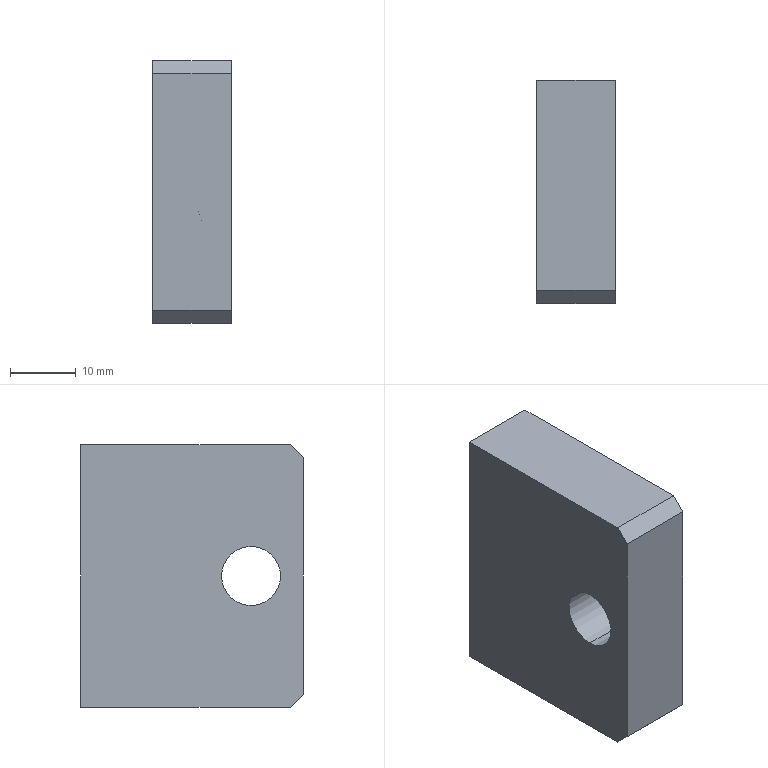Part | STEP file | PN_0024 | 1 solid | 24 faces | box 12 x 34 x 40 mm | volume 15028 mm3 | cylinder 10 | plane 10 | cone 4 | commonest cylinder face diameters 4 x4 4.2 x4 9 x2